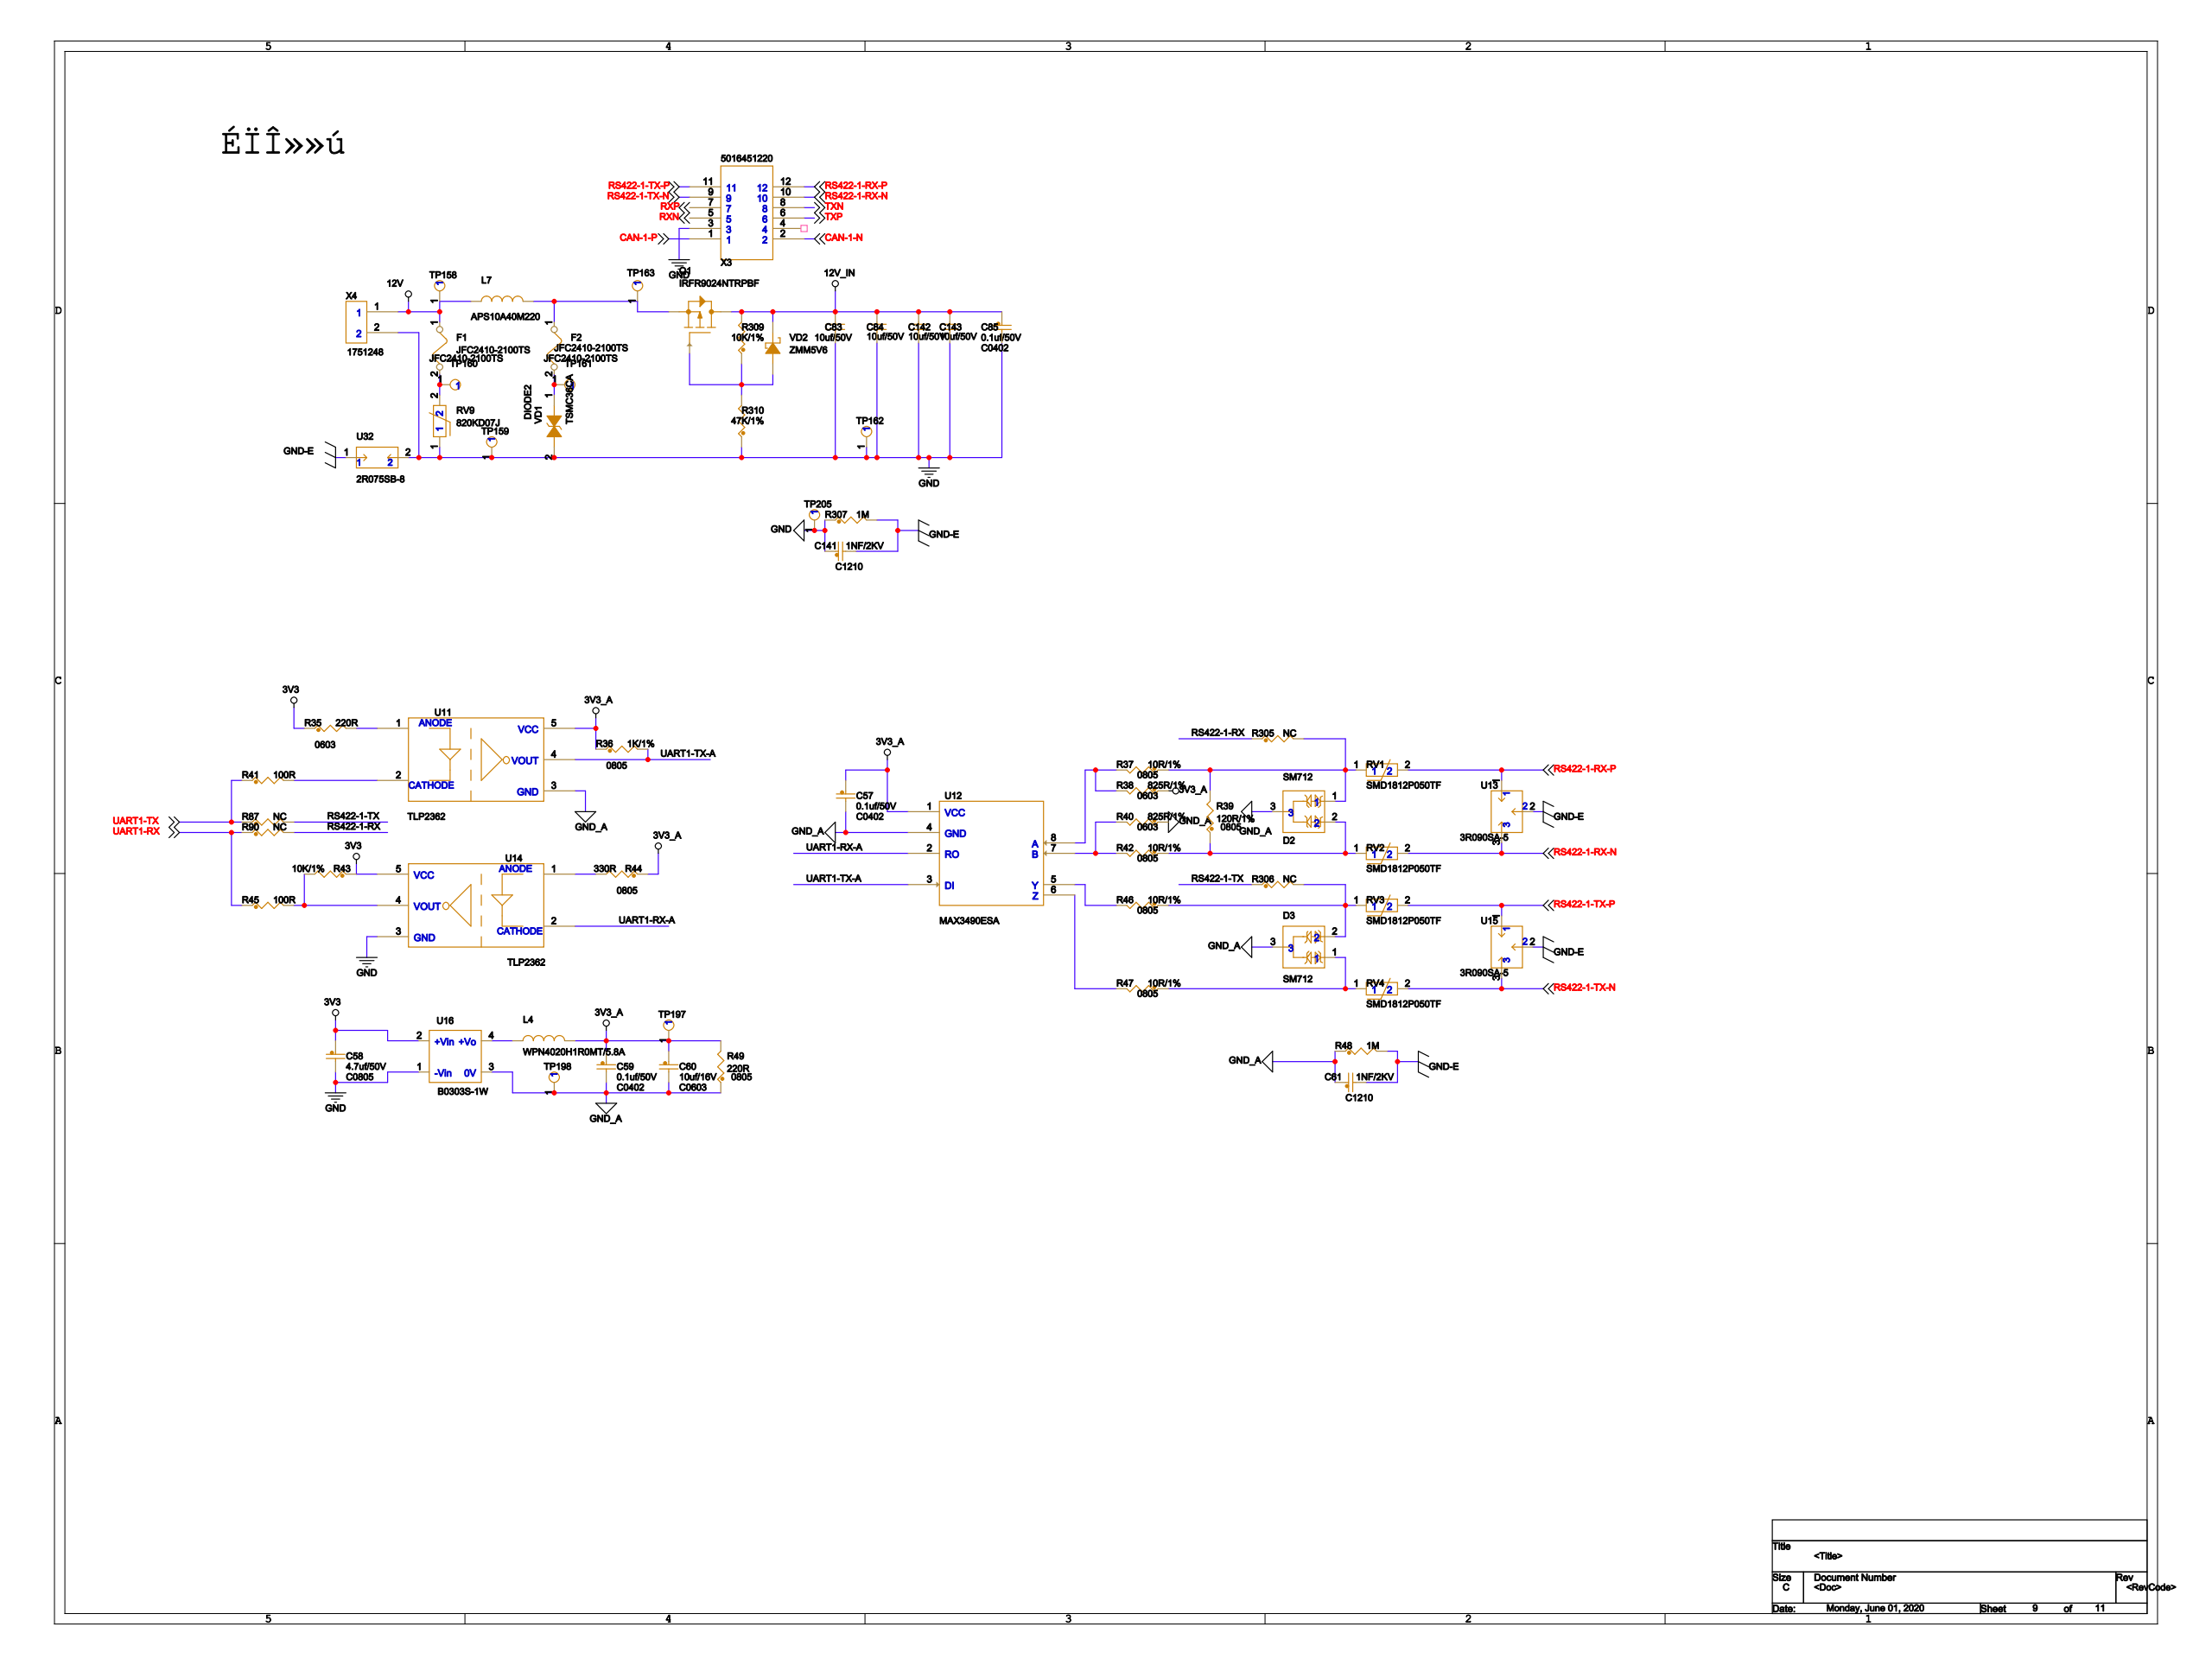Circuit board | Cadence Allegro | 792 parts | 400 nets | one sheet of the schematic
Parts on this sheet (reference | value | footprint):
C57 | 0.1uf/50V | C0402
C58 | 4.7uf/50V | C0805
C59 | 0.1uf/50V | C0402
C60 | 10uf/16V | C0603
C61 | 1NF/2KV | C1210
C83 | 10uf/50V | C0805
C84 | 10uf/50V | C0805
C85 | 0.1uf/50V | C0402
C141 | 1NF/2KV | C1210
C142 | 10uf/50V | C0805
C143 | 10uf/50V | C0805
D2 | SM712 | SOT23
D3 | SM712 | SOT23
F1 | JFC2410-2100TS | JFC2410-2100TS
F2 | JFC2410-2100TS | JFC2410-2100TS
L4 | WPN4020H1R0MT/5.8A | SM_IND_4
L7 | APS10A40M220 | SM_IND_10X10
Q1 | IRFR9024NTRPBF | TO252-2
R35 | 220R | 0603
R36 | 1K/1% | 0805
R37 | 10R/1% | 0805
R38 | 825R/1% | 0603
R39 | 120R/1% | 0805
R40 | 825R/1% | 0603
R41 | 100R | 0603
R42 | 10R/1% | 0805
R43 | 10K/1% | 0402
R44 | 330R | 0805
R45 | 100R | 0603
R46 | 10R/1% | 0805
R47 | 10R/1% | 0805
R48 | 1M | 1206
R49 | 220R | 0805
R87 | NC | 0603
R90 | NC | 0603
R305 | NC | 0603
R306 | NC | 0603
R307 | 1M | 1206
R309 | 10K/1% | 0603
R310 | 47K/1% | 0603
RV1 | SMD1812P050TF | 1812_2
RV2 | SMD1812P050TF | 1812_2
RV3 | SMD1812P050TF | 1812_2
RV4 | SMD1812P050TF | 1812_2
RV9 | 820KD07J | 10D151K
TP158 | TESTPOINT | TESTPOINT-33MIL
TP159 | TESTPOINT | TESTPOINT-33MIL
TP160 | TESTPOINT | TESTPOINT-33MIL
TP161 | TESTPOINT | TESTPOINT-33MIL
TP162 | TESTPOINT | TESTPOINT-33MIL
TP163 | TESTPOINT | TESTPOINT-33MIL
TP197 | TESTPOINT | TESTPOINT-33MIL
TP198 | TESTPOINT | TESTPOINT-33MIL
TP205 | TESTPOINT | TESTPOINT-33MIL
U11 | TLP2362 | TLP2362
U12 | MAX3490ESA | SOP8
U13 | 3R090SA-5 | 3R090SA-5
U14 | TLP2362 | TLP2362
U15 | 3R090SA-5 | 3R090SA-5
U16 | B0303S-1W | B0303S
U32 | 2R075SB-8 | 2R075SB
VD2 | ZMM5V6 | DIODE2
X3 | 5016451220 | 5016451220
X4 | 1751248 | EDG-35-2P
Nets of these parts (net: part-pin ...):
3V3: C58-1 R35-1 R43-1 U14-5 U16-2
GND-E: C61-2 C141-2 R48-2 R307-2 U13-2 U15-2 U32-1
GND: C58-2 C83-2 C84-2 C85-2 C141-1 C142-2 C143-2 R307-1 R310-1 RV9-1 TP159-1 TP162-1 TP205-1 U14-3 U16-1 U32-2 X3-3 X4-2
CAN-1-P: X3-1
RS422-1-RX-N: RV2-2 U13-3 X3-10
RS422-1-TX-P: RV3-2 U15-1 X3-11
RS422-1-RX-P: RV1-2 U13-1 X3-12
CAN-1-N: X3-2
RXN: X3-5
TXP: X3-6
RXP: X3-7
TXN: X3-8
RS422-1-TX-N: RV4-2 U15-3 X3-9
12V: F1-1 L7-1 TP158-1 X4-1
N7979189: F2-1 L7-2 Q1-2 TP163-1
12V_IN: C83-1 C84-1 C85-1 C142-1 C143-1 Q1-3 R309-2 VD2-2
N7979213: Q1-1 R309-1 R310-2 VD2-1
N7979029: F1-2 RV9-2 TP160-1
3V3_A: C57-1 C59-1 C60-1 L4-2 R36-1 R38-1 R44-1 R49-2 TP197-1 U11-5 U12-1
GND_A: C57-2 C59-2 C60-2 C61-1 D2-3 D3-3 R40-1 R48-1 R49-1 TP198-1 U11-3 U12-4 U16-3
N7979061: F2-2 TP161-1
N8066949: R35-2 U11-1
UART1-TX: R41-1 R87-1
N8066953: R41-2 U11-2
UART1-RX: R45-1 R90-1
N8067003: R43-2 R45-2 U14-4
UART1-TX-A: R36-2 U11-4 U12-3
N8065945: R37-2 R38-2 U12-8
N8065949: R40-2 R42-2 U12-7
N8067087: R44-2 U14-1
UART1-RX-A: U12-2 U14-2
N8066057: D2-1 R37-1 R39-2 R305-2 RV1-1
N8066061: D2-2 R39-1 R42-1 RV2-1
N8066267: D3-1 R47-1 RV4-1
N8066347: D3-2 R46-1 R306-2 RV3-1
N8067395: L4-1 U16-4
N8066675: R46-2 U12-5
N8066683: R47-2 U12-6
RS422-1-RX: R90-2 R305-1
RS422-1-TX: R87-2 R306-1